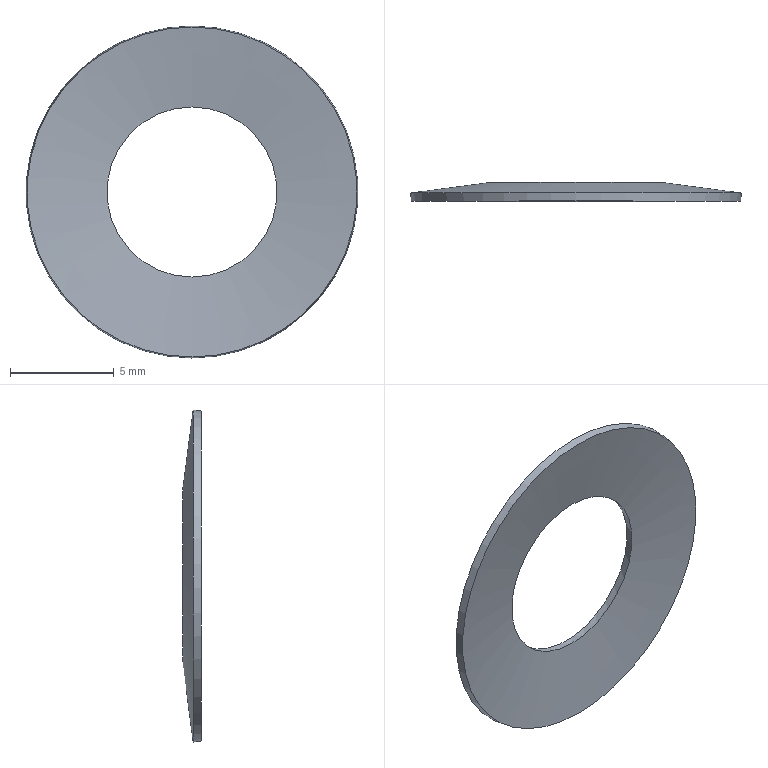Part | STEP file | Disc spring | 1 solid | 4 faces | box 16 x 0.9 x 16 mm | volume 59.01 mm3 | cone 4
STEP:
#1=CARTESIAN_POINT('',(0.,0.9,4.152));
#2=VERTEX_POINT('',#1);
#3=CARTESIAN_POINT('',(0.,0.9,0.));
#4=DIRECTION('',(0.,1.,0.));
#5=DIRECTION('',(0.,0.,1.));
#6=AXIS2_PLACEMENT_3D('',#3,#4,#5);
#7=CIRCLE('',#6,4.152);
#8=EDGE_CURVE('',#2,#2,#7,.T.);
#9=ORIENTED_EDGE('',*,*,#8,.F.);
#10=EDGE_LOOP('',(#9));
#11=FACE_OUTER_BOUND('',#10,.T.);
#12=CARTESIAN_POINT('',(0.,0.3966,8.));
#13=VERTEX_POINT('',#12);
#14=CARTESIAN_POINT('',(0.,0.3966,0.));
#15=DIRECTION('',(0.,1.,0.));
#16=DIRECTION('',(0.,0.,1.));
#17=AXIS2_PLACEMENT_3D('',#14,#15,#16);
#18=CIRCLE('',#17,8.);
#19=EDGE_CURVE('',#13,#13,#18,.T.);
#20=ORIENTED_EDGE('',*,*,#19,.T.);
#21=EDGE_LOOP('',(#20));
#22=FACE_OUTER_BOUND('',#21,.T.);
#23=CARTESIAN_POINT('',(0.,0.6483,0.));
#24=DIRECTION('',(0.,-1.,0.));
#25=DIRECTION('',(0.,0.,-1.));
#26=AXIS2_PLACEMENT_3D('',#23,#24,#25);
#27=CONICAL_SURFACE('',#26,6.076,1.441);
#28=ADVANCED_FACE('',(#11,#22),#27,.T.);
#29=ORIENTED_EDGE('',*,*,#19,.F.);
#30=EDGE_LOOP('',(#29));
#31=FACE_OUTER_BOUND('',#30,.T.);
#32=CARTESIAN_POINT('',(0.,0.,7.948));
#33=VERTEX_POINT('',#32);
#34=CARTESIAN_POINT('',(0.,0.,0.));
#35=DIRECTION('',(0.,1.,0.));
#36=DIRECTION('',(0.,0.,1.));
#37=AXIS2_PLACEMENT_3D('',#34,#35,#36);
#38=CIRCLE('',#37,7.948);
#39=EDGE_CURVE('',#33,#33,#38,.T.);
#40=ORIENTED_EDGE('',*,*,#39,.T.);
#41=EDGE_LOOP('',(#40));
#42=FACE_OUTER_BOUND('',#41,.T.);
#43=CARTESIAN_POINT('',(0.,0.1983,0.));
#44=DIRECTION('',(0.,1.,0.));
#45=DIRECTION('',(0.,0.,1.));
#46=AXIS2_PLACEMENT_3D('',#43,#44,#45);
#47=CONICAL_SURFACE('',#46,7.974,0.1301);
#48=ADVANCED_FACE('',(#31,#42),#47,.T.);
#49=CARTESIAN_POINT('',(0.,0.5034,4.1));
#50=VERTEX_POINT('',#49);
#51=CARTESIAN_POINT('',(0.,0.5034,0.));
#52=DIRECTION('',(0.,1.,0.));
#53=DIRECTION('',(0.,0.,1.));
#54=AXIS2_PLACEMENT_3D('',#51,#52,#53);
#55=CIRCLE('',#54,4.1);
#56=EDGE_CURVE('',#50,#50,#55,.T.);
#57=ORIENTED_EDGE('',*,*,#56,.T.);
#58=EDGE_LOOP('',(#57));
#59=FACE_OUTER_BOUND('',#58,.T.);
#60=ORIENTED_EDGE('',*,*,#39,.F.);
#61=EDGE_LOOP('',(#60));
#62=FACE_OUTER_BOUND('',#61,.T.);
#63=CARTESIAN_POINT('',(0.,0.2517,0.));
#64=DIRECTION('',(0.,-1.,0.));
#65=DIRECTION('',(0.,0.,-1.));
#66=AXIS2_PLACEMENT_3D('',#63,#64,#65);
#67=CONICAL_SURFACE('',#66,6.024,1.441);
#68=ADVANCED_FACE('',(#59,#62),#67,.F.);
#69=ORIENTED_EDGE('',*,*,#8,.T.);
#70=EDGE_LOOP('',(#69));
#71=FACE_OUTER_BOUND('',#70,.T.);
#72=ORIENTED_EDGE('',*,*,#56,.F.);
#73=EDGE_LOOP('',(#72));
#74=FACE_OUTER_BOUND('',#73,.T.);
#75=CARTESIAN_POINT('',(0.,0.7017,0.));
#76=DIRECTION('',(0.,1.,0.));
#77=DIRECTION('',(0.,0.,1.));
#78=AXIS2_PLACEMENT_3D('',#75,#76,#77);
#79=CONICAL_SURFACE('',#78,4.126,0.1301);
#80=ADVANCED_FACE('',(#71,#74),#79,.F.);
#81=CLOSED_SHELL('',(#28,#48,#68,#80));
#82=MANIFOLD_SOLID_BREP('',#81);
#83=(LENGTH_UNIT()NAMED_UNIT(*)SI_UNIT(.MILLI.,.METRE.));
#84=UNCERTAINTY_MEASURE_WITH_UNIT(LENGTH_MEASURE(0.00001),#83,'','');
#85=(NAMED_UNIT(*)PLANE_ANGLE_UNIT()SI_UNIT($,.RADIAN.));
#86=(NAMED_UNIT(*)SI_UNIT($,.STERADIAN.)SOLID_ANGLE_UNIT());
#87=(GEOMETRIC_REPRESENTATION_CONTEXT(3)GLOBAL_UNCERTAINTY_ASSIGNED_CONTEXT((#84))GLOBAL_UNIT_ASSIGNED_CONTEXT((#83,#85,#86))REPRESENTATION_CONTEXT('',''));
#88=ADVANCED_BREP_SHAPE_REPRESENTATION('',(#82),#87);